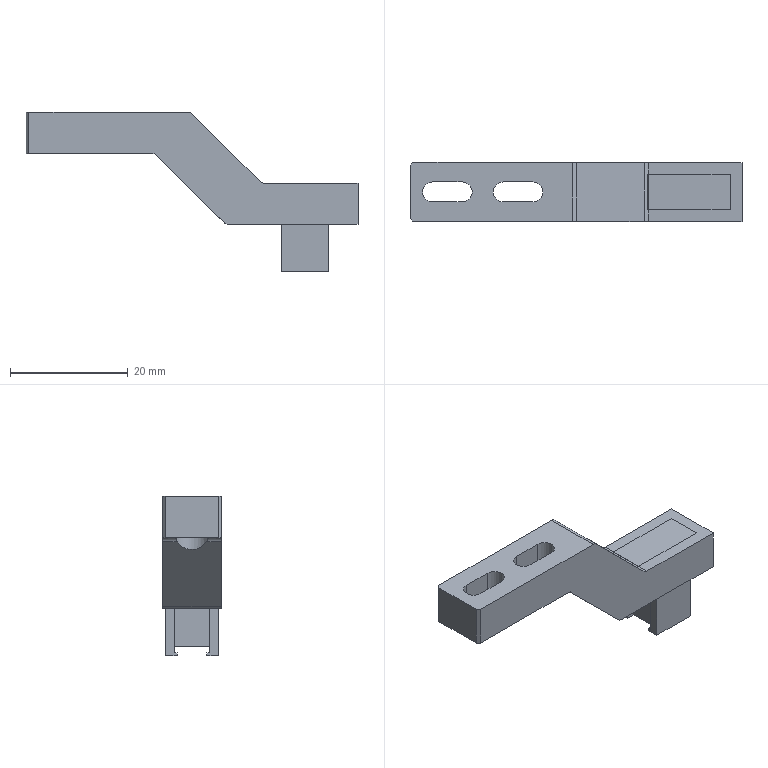NC program | NX | posted with a generic post | part box 56.3 x 10 x 27 mm
Lines 1 to 981 of 3920:
N10 G17 G21 G94 G90
(FLOOR_WALL_COPY , TOOL : D63)
N12 T01 M6
N14 G54
N16 G17 G0 G90 X62.65 Y0. S6500 M3
N18 G43 Z30. H1
N20 Z5.
N22 G94 G1 Z2. F1250.
N24 X59.65
N26 X-59.65
N28 X-62.65
N30 Z5.
N32 G0 Z30.
N34 X62.65
N36 Z4.
N38 G1 Z1.
N40 X59.65
N42 X-59.65
N44 X-62.65
N46 Z4.
N48 G0 Z30.
N50 X62.65
N52 Z3.
N54 G1 Z0.
N56 X59.65
N58 X-59.65
N60 X-62.65
N62 Z3.
N64 G0 Z30.
N66 M5
(ADAPTIVE_MILLING_COPY , TOOL : D10)
N68 T10 M6
N70 G54
N72 G17 G0 G90 X-29.095 Y-12.49 S9500 M3
N74 G43 Z30. H10
N76 Z-19.
N78 G94 G1 Z-20. F1000.
N80 X-28.723 Y-11.01 F3000.
N82 G3 X-29.383 Y-9.805 R1.015
N84 G2 X-31.661 Y-8.267 R5.47
N86 G1 X-32.538 Y-7.171
N88 X-32.612 Y-7.045
N90 X-32.995 Y-6.121
N92 G3 X-34.101 Y-5.513 R1.017
N94 G1 X-35.635 Y-5.779
N96 Z-17.
N98 G0 Z30.
N100 X-35.645 Y5.809
N102 Z-19.
N104 G1 Z-20. F1000.
N106 X-34.099 Y5.532 F3000.
N108 G3 X-32.988 Y6.14 R1.017
N110 G1 X-32.612 Y7.046
N112 X-32.539 Y7.17
N114 G2 X-30.75 Y9.106 R10.067
N116 X-29.382 Y9.805 R5.529
N118 G3 X-28.721 Y11.01 R1.015
N120 G1 X-29.093 Y12.485
N122 Z-17.
N124 G0 Z30.
N126 X-7.082 Y-12.562
N128 Z-18.85
N130 G1 Z-19.85 F1000.
N132 X-6.916 Y-11.769 F3000.
N134 X-6.774 Y-10.97
N136 G3 X-7.457 Y-9.975 R1.017
N138 X-11.391 Y-9.343 R13.467
N140 X-25.489 Y-9.186 R390.39
N142 G2 X-30.036 Y-6.459 R5.899
N144 X-31.966 Y-0.735 R12.739
N146 X-32.139 Y2.952 R16.321
N148 X-29.051 Y7.174 R6.209
N150 X-23.245 Y8.879 R13.977
N152 X-12.954 Y9.183 R112.101
N154 G3 X-9.257 Y9.221 R59.444
N156 G2 X-7.427 Y9.998 R15.276
N158 G3 X-7.037 Y11.746 R1.002
N160 X-7.789 Y11.981 Z-19.81 R1.212
N162 G1 X-8.981 Y12.072 Z-19.75
N164 X-11.324 Y12.248
N166 X-19.449
N168 G3 X-25.626 Y11.575 R29.031
N170 G1 X-26.698 Y11.337
N172 X-27.758 Y11.048
N174 G3 X-30.519 Y9.807 R13.655
N176 G1 X-32.085 Y8.865
N178 G3 X-33.546 Y7.281 R4.683
N180 G1 X-34.64 Y5.273
N182 G3 X-35.27 Y2.811 R6.964
N184 X-35.265 Y0.821 R11.97
N186 G1 X-35.027 Y-1.664
N188 G3 X-32.575 Y-7.973 R14.447
N190 G1 X-31.861 Y-8.997
N192 X-31.107 Y-9.991
N194 G3 X-30.156 Y-10.765 R3.251
N196 X-27.286 Y-11.946 R11.99
N198 X-24.825 Y-12.314 R13.023
N200 G1 X-11.112 Y-12.996
N202 X-10.881 Y-12.977
N204 X-10.659 Y-12.912
N206 X-8.91 Y-12.142
N208 X-8.301 Y-11.879 Z-19.783
N210 X-7.702 Y-11.595 Z-19.816
N212 G3 X-7.302 Y-11.069 Z-19.85 R1.04
N214 X-7.93 Y-9.814 R1.005
N216 G2 X-9.405 Y-9.206 R53.931
N218 G3 X-14.448 Y-8.54 R21.088
N220 X-23.346 Y-8.378 R966.397
N222 G2 X-29.253 Y-4.402 R7.758
N224 X-30.713 Y0.018 R9.774
N226 X-27.658 Y5.685 R6.887
N228 X-21.61 Y7.889 R13.615
N230 X-13.229 Y8.35 R64.733
N232 G3 X-10.141 Y8.517 R15.214
N234 X-8.908 Y9.377 R10.818
N236 X-8.643 Y10.699 R1.005
N238 X-9.549 Y11.199 Z-19.796 R1.107
N240 G1 X-10.461 Y11.321 Z-19.75
N242 X-12.805 Y11.627
N244 X-16.819 Y11.613
N246 G3 X-22.105 Y10.949 R28.919
N248 G1 X-24.626 Y10.376
N250 G3 X-29.545 Y8.323 R20.292
N252 X-32.51 Y5.291 R8.578
N254 X-33.55 Y2.864 R10.425
N256 X-33.946 Y1.048 R9.738
N258 X-33.405 Y-2.601 R8.322
N260 G1 X-32.84 Y-4.095
N262 X-32.26 Y-5.583
N264 G3 X-30.444 Y-8.234 R8.852
N266 X-29.053 Y-9.465 R9.477
N268 G1 X-28.528 Y-9.786
N270 X-27.98 Y-10.064
N272 G3 X-25.183 Y-11.114 R24.495
N274 X-23.224 Y-11.415 R8.92
N276 G1 X-12.474 Y-11.804
N278 X-12.318 Y-11.798
N280 X-10.15 Y-11.536
N282 X-9.486 Y-11.46 Z-19.783
N284 X-8.825 Y-11.362 Z-19.817
N286 G3 X-8.294 Y-10.985 Z-19.85 R1.041
N288 X-8.577 Y-9.554 R1.004
N290 X-12.565 Y-8.09 R8.471
N292 X-20.747 Y-7.642 R67.984
N294 G2 X-28.031 Y-3.29 R8.284
N296 X-27.114 Y3.185 R6.128
N298 X-21.759 Y6.499 R10.353
N300 X-14.338 Y7.453 R31.44
N302 G3 X-10.767 Y7.816 R15.161
N304 X-9.893 Y8.632 R2.14
N306 G1 X-9.821 Y8.701
N308 G3 X-9.629 Y9.891 R1.007
N310 X-10.436 Y10.425 Z-19.8 R1.037
N312 G1 X-11.413 Y10.597 Z-19.75
N314 X-13.396 Y10.947
N316 X-13.557 Y10.958
N318 X-13.718 Y10.951
N320 X-21.538 Y9.776
N322 G3 X-25.619 Y8.334 R11.544
N324 X-30.189 Y4.197 R14.319
N326 G1 X-30.651 Y3.515
N328 X-31.071 Y2.807
N330 G3 X-31.699 Y-0.315 R5.897
N332 G1 X-31.595 Y-1.716
N334 X-31.471 Y-3.116
N336 G3 X-30.853 Y-4.752 R4.789
N338 G1 X-30.104 Y-5.877
N340 X-29.329 Y-6.984
N342 G3 X-27.033 Y-8.977 R8.046
N344 X-23.3 Y-10.28 R10.192
N346 X-17.104 Y-10.992 R86.895
N348 G1 X-13.208 Y-11.279
N350 X-11.031 Y-10.969
N352 X-10.377 Y-10.88 Z-19.783
N354 X-9.728 Y-10.766 Z-19.816
N356 G3 X-9.198 Y-10.359 Z-19.85 R1.039
N358 X-9.42 Y-9.027 R1.005
N360 X-12.364 Y-7.611 R5.895
N362 X-19.018 Y-6.918 R38.53
N364 G2 X-23.754 Y-5.513 R9.337
N366 X-25.428 Y0.573 R5.13
N368 X-21.1 Y4.933 R8.141
N370 X-15.011 Y6.433 R19.241
N372 G3 X-11.371 Y7.051 R17.404
N374 X-10.667 Y7.667 R1.259
N376 G1 X-10.292 Y8.135
N378 G3 X-10.2 Y9.25 R1.01
N380 X-10.945 Y9.757 Z-19.803 R1.047
N382 G1 X-11.986 Y9.994 Z-19.75
N384 X-12.93 Y10.215
N386 X-13.879 Y10.412
N388 X-14.189 Y10.385
N390 X-17.418 Y9.565
N392 G3 X-23.015 Y7.362 R30.115
N394 X-25.904 Y5.324 R13.843
N396 X-27.531 Y3.25 R9.668
N398 G1 X-28.137 Y2.209
N400 X-28.726 Y1.158
N402 G3 X-29.135 Y-1.686 R4.979
N404 X-28.711 Y-3.27 R6.554
N406 G1 X-28.229 Y-4.44
N408 X-27.73 Y-5.603
N410 G3 X-24.517 Y-8.671 R6.669
N412 X-22.152 Y-9.426 R10.665
N414 G1 X-13.426 Y-11.085
N416 X-13.181 Y-11.071
N418 X-11.297 Y-10.727
N420 X-10.648 Y-10.614 Z-19.783
N422 X-10.003 Y-10.477 Z-19.816
N424 G3 X-9.489 Y-10.05 Z-19.85 R1.039
N426 X-9.651 Y-8.82 R1.007
N428 X-12.954 Y-6.968 R6.175
N430 X-18.092 Y-6.206 R37.578
N432 G2 X-21.119 Y-4.858 R4.47
N434 X-21.743 Y0.226 R4.837
N436 X-17.592 Y4.231 R8.054
N438 X-12.947 Y5.775 R33.71
N440 G3 X-11.176 Y6.658 R4.145
N442 X-10.738 Y7.55 R7.192
N444 X-10.92 Y8.632 R1.01
N446 X-11.892 Y8.942 Z-19.797 R1.115
N448 G1 X-12.828 Y8.893 Z-19.75
N450 X-14.861 Y8.78
N452 X-15.085 Y8.715
N454 G3 X-20.073 Y6.318 R44.561
N456 X-23.345 Y3.452 R11.589
N458 G1 X-24.168 Y2.369
N460 G3 X-25.085 Y-0.66 R5.509
N462 X-23.769 Y-5.511 R9.449
N464 X-21.913 Y-7.647 R9.299
N466 X-17.768 Y-9.753 R8.705
N468 G1 X-15.897 Y-10.136
N470 X-14.022 Y-10.496
N472 X-13.749 Y-10.475
N474 X-11.973 Y-10.091
N476 X-11.316 Y-9.953 Z-19.784
N478 X-10.664 Y-9.793 Z-19.817
N480 G3 X-10.173 Y-9.374 Z-19.85 R1.041
N482 X-10.261 Y-8.229 R1.007
N484 X-12.616 Y-6.595 R4.561
N486 X-15.415 Y-5.848 R27.634
N488 G2 X-17.591 Y-2.639 R3.565
N490 X-15.665 Y2.136 R6.397
N492 X-12.32 Y4.826 R24.044
N494 G3 X-11.366 Y5.826 R2.693
N496 G2 X-11.035 Y6.875 R3.828
N498 G3 X-11.436 Y8.135 R1.005
N500 X-12.403 Y8.175 Z-19.8 R1.037
N502 G1 X-13.328 Y7.818 Z-19.75
N504 X-14.324 Y7.438
N506 X-15.314 Y7.042
N508 X-15.535 Y6.875
N510 X-16.742 Y5.673
N512 X-17.934 Y4.456
N514 G3 X-19.803 Y1.357 R9.754
N516 G1 X-20.095 Y0.566
N518 X-20.341 Y-0.241
N520 G3 X-20.431 Y-2.92 R6.368
N522 X-19.976 Y-4.243 R5.551
N524 G1 X-19.325 Y-5.556
N526 X-18.653 Y-6.859
N528 G3 X-16.386 Y-8.672 R4.213
N530 G1 X-14.631 Y-9.247
N532 X-12.462 Y-9.477
N534 X-11.811 Y-9.549 Z-19.783
N536 X-11.159 Y-9.596 Z-19.816
N538 G3 X-10.539 Y-9.323 Z-19.85 R1.038
N540 X-10.39 Y-8.054 R1.007
N542 X-12.253 Y-6.296 R4.463
N544 G2 X-14.109 Y-1.889 R4.864
N546 X-12.538 Y2.385 R9.455
N548 G3 X-11.5 Y4.204 R10.631
N550 G2 X-11.315 Y6.023 R12.347
N552 G3 X-12.598 Y7.131 R1.002
N554 X-13.233 Y6.59 Z-19.807 R1.173
N556 G1 X-13.887 Y5.65 Z-19.75
N558 X-15.152 Y3.839
N560 X-15.821 Y3.15
N562 G3 X-16.324 Y2.308 R3.162
N564 X-17.074 Y-0.188 R11.037
N566 G1 X-17.333 Y-2.504
N568 X-17.567 Y-4.822
N570 G3 X-16.464 Y-6.889 R2.105
N572 G1 X-15.156 Y-7.58
N574 X-13.093 Y-8.503
N576 X-12.46 Y-8.789 Z-19.785
N578 X-11.82 Y-9.059 Z-19.82
N580 G3 X-11.22 Y-9.037 Z-19.85 R1.047
N582 X-10.716 Y-7.551 R1.003
N584 G2 X-12.171 Y-4.447 R9.788
N586 X-11.741 Y0.772 R10.008
N588 G3 X-11.396 Y2.055 R6.869
N590 G2 X-11.474 Y4.376 R17.958
N592 G3 X-13.672 Y4.322 R-1.1
N594 G1 X-13.081 Y-7.6
N596 G3 X-10.95 Y-7.167 R-1.1
N598 G2 X-11.474 Y-4.966 R6.015
N600 X-10.997 Y0.064 R17.199
N602 G3 X-11.006 Y0.742 R1.809
N604 G2 X-11.401 Y2.103 R3.769
N606 G3 X-13.596 Y1.974 R1.1
N608 G1 X-13.529 Y-1.466
N610 G3 X-11.359 Y-1.699 R1.1
N612 G1 X-11.326 Y-1.56
N614 X-10.929 Y-0.538
N616 X-10.891 Y-0.419
N618 X-10.849 Y-0.257
N620 G3 X-11.04 Y0.83 R1.782
N622 X-12.218 Y1.443 R1.015
N624 G1 X-13.775 Y1.068
N626 Z-16.85
N628 G0 Z30.
N630 X-6.934 Y-12.51
N632 Z-18.403
N634 G1 Z-19.403 F1000.
N636 X-6.755 Y-11.705 F3000.
N638 X-6.598 Y-10.895
N640 G3 X-7.221 Y-9.903 R1.017
N642 G2 X-10.204 Y-7.513 R5.363
N644 X-10.871 Y-4.965 R6.053
N646 X-10.737 Y-1.404 R21.01
N648 G3 X-10.761 Y1.513 R4.162
N650 G2 X-10.703 Y6.266 R17.594
N652 X-8.225 Y9.488 R5.424
N654 G1 X-7.116 Y9.946
N656 G3 X-7.6 Y11.865 R1.
N658 G1 X-9.58 Y11.582 Z-19.303
N660 X-10.319 Y11.482
N662 X-11.054 Y11.358
N664 X-11.271 Y11.256
N666 X-11.462 Y11.111
N668 X-11.902 Y10.672
N670 X-12.298 Y10.194
N672 X-12.456 Y9.929
N674 X-12.597 Y9.655
N676 X-13.458 Y7.659
N678 G3 X-14.312 Y3.881 R13.264
N680 G1 X-14.508 Y1.226
N682 G3 X-14.201 Y0.429 R1.016
N684 G1 X-13.127 Y-0.596
N686 X-12.634 Y-1.071 Z-19.337
N688 X-12.128 Y-1.532 Z-19.372
N690 G3 X-11.533 Y-1.709 Z-19.403 R1.044
N692 X-10.61 Y-1.024 R1.007
N694 X-10.397 Y0.36 R2.262
N696 G1 X-10.426 Y0.468
N698 X-10.584 Y0.942
N700 G3 X-11.815 Y1.596 R1.015
N702 G1 X-13.23 Y1.199
N704 Z-16.403
N706 G0 Z30.
N708 X-5.663 Y-12.6
N710 Z-17.806
N712 G1 Z-18.806 F1000.
N714 X-5.955 Y-10.725 F3000.
N716 G3 X-6.572 Y-9.945 R1.024
N718 G2 X-10.178 Y-6.271 R5.329
N720 G1 X-10.348 Y-5.036
N722 X-10.353 Y-4.964
N724 G2 X-10.256 Y-1.202 R28.314
N726 G3 X-10.269 Y1.277 R3.928
N728 G2 X-10.348 Y5.036 R30.281
N730 X-8.856 Y8.6 R5.576
N732 X-6.562 Y9.95 R5.798
N734 G3 X-7.063 Y11.868 R1.
N736 G1 X-9.043 Y11.584 Z-18.706
N738 X-9.773 Y11.484
N740 X-10.5 Y11.362
N742 X-10.717 Y11.26
N744 X-10.908 Y11.114
N746 X-11.348 Y10.675
N748 X-11.745 Y10.198
N750 X-11.904 Y9.934
N752 X-12.047 Y9.66
N754 X-12.953 Y7.59
N756 G3 X-13.817 Y3.884 R13.572
N758 G1 X-14.011 Y1.631
N760 G3 X-13.722 Y0.837 R1.024
N762 G1 X-12.634 Y-0.25
N764 X-12.16 Y-0.731 Z-18.74
N766 X-11.67 Y-1.196 Z-18.774
N768 G3 X-11.061 Y-1.383 Z-18.806 R1.042
N770 X-10.114 Y-0.619 R1.007
N772 X-10.072 Y0.442 R1.7
N774 X-11.066 Y1.213 R1.017
N776 G1 X-12.768 Y1.192
N778 Z-15.806
N780 G0 Z30.
N782 X-5.041 Y-12.603
N784 Z-17.21
N786 G1 Z-18.21 F1000.
N788 X-5.339 Y-10.729 F3000.
N790 G3 X-5.955 Y-9.952 R1.024
N792 G2 X-9.07 Y-7.522 R5.482
N794 X-9.753 Y-4.964 R6.077
N796 G1 Y-1.39
N798 X-9.75 Y-1.332
N800 G3 X-9.753 Y1.306 R7.407
N802 G1 Y4.964
N804 X-9.748 Y5.036
N806 G2 X-8.256 Y8.6 R5.576
N808 X-5.948 Y9.955 R5.84
N810 G3 X-6.456 Y11.873 R1.
N812 G1 X-8.436 Y11.588 Z-18.11
N814 X-9.163 Y11.489
N816 X-9.886 Y11.367
N818 X-10.103 Y11.265
N820 X-10.295 Y11.12
N822 X-11.04 Y10.378
N824 X-11.772 Y9.624
N826 G3 X-12.809 Y6.852 R4.345
N828 G1 X-12.835 Y2.52
N830 X-12.774 Y2.276
N832 X-12.234 Y0.883
N834 X-11.543 Y-0.882 Z-18.204
N836 X-11.491 Y-0.972 Z-18.21
N838 G3 X-9.66 Y-0.537 R1.001
N840 X-9.626 Y0.221 R7.411
N842 X-10.714 Y1.107 R1.015
N844 G1 X-12.235 Y0.978
N846 Z-15.21
N848 G0 Z30.
N850 X-4.441 Y-12.603
N852 Z-16.613
N854 G1 Z-17.613 F1000.
N856 X-4.739 Y-10.729 F3000.
N858 G3 X-5.355 Y-9.952 R1.024
N860 G2 X-8.47 Y-7.522 R5.482
N862 X-9.153 Y-4.964 R6.077
N864 G1 Y4.964
N866 X-9.148 Y5.036
N868 G2 X-7.656 Y8.6 R5.576
N870 X-5.348 Y9.955 R5.84
N872 G3 X-4.738 Y11.085 R1.017
N874 G1 X-5.02 Y12.525
N876 Z-14.613
N878 G0 Z30.
N880 X-3.841 Y-12.603
N882 Z-16.016
N884 G1 Z-17.016 F1000.
N886 X-4.139 Y-10.729 F3000.
N888 G3 X-4.755 Y-9.952 R1.024
N890 G2 X-7.87 Y-7.522 R5.482
N892 X-8.553 Y-4.964 R6.077
N894 G1 Y4.964
N896 X-8.548 Y5.036
N898 G2 X-7.056 Y8.599 R5.576
N900 X-4.748 Y9.955 R5.84
N902 G3 X-4.138 Y11.085 R1.017
N904 G1 X-4.42 Y12.525
N906 Z-14.016
N908 G0 Z30.
N910 X-3.241 Y-12.603
N912 Z-15.419
N914 G1 Z-16.419 F1000.
N916 X-3.539 Y-10.729 F3000.
N918 G3 X-4.155 Y-9.952 R1.024
N920 G2 X-7.27 Y-7.522 R5.481
N922 X-7.953 Y-4.964 R6.077
N924 G1 Y4.964
N926 X-7.948 Y5.036
N928 G2 X-6.456 Y8.6 R5.576
N930 X-4.147 Y9.955 R5.84
N932 G3 X-3.537 Y11.085 R1.017
N934 G1 X-3.819 Y12.525
N936 Z-13.419
N938 G0 Z30.
N940 X-2.641 Y-12.603
N942 Z-14.823
N944 G1 Z-15.823 F1000.
N946 X-2.939 Y-10.729 F3000.
N948 G3 X-3.555 Y-9.952 R1.024
N950 G2 X-6.67 Y-7.522 R5.481
N952 X-7.352 Y-4.964 R6.077
N954 G1 Y4.964
N956 X-7.348 Y5.036
N958 G2 X-5.856 Y8.599 R5.576
N960 X-3.547 Y9.955 R5.84
N962 G3 X-2.937 Y11.085 R1.017
N964 G1 X-3.219 Y12.525
N966 Z-12.823
N968 G0 Z30.
N970 X-2.042 Y-12.603
N972 Z-14.226
N974 G1 Z-15.226 F1000.
N976 X-2.339 Y-10.729 F3000.
N978 G3 X-2.955 Y-9.952 R1.024
N980 G2 X-6.07 Y-7.522 R5.481
N982 X-6.752 Y-4.964 R6.077
N984 G1 Y4.964
N986 X-6.747 Y5.036
N988 G2 X-5.256 Y8.599 R5.576
N990 X-2.947 Y9.955 R5.84
N992 G3 X-2.337 Y11.085 R1.017
N994 G1 X-2.619 Y12.525
N996 Z-12.226
N998 G0 Z30.
N1000 X-1.442 Y-12.603
N1002 Z-13.629
N1004 G1 Z-14.629 F1000.
N1006 X-1.739 Y-10.729 F3000.
N1008 G3 X-2.355 Y-9.952 R1.024
N1010 G2 X-5.469 Y-7.522 R5.481
N1012 X-6.152 Y-4.964 R6.077
N1014 G1 Y4.964
N1016 X-6.147 Y5.036
N1018 G2 X-4.655 Y8.599 R5.576
N1020 X-2.347 Y9.955 R5.84
N1022 G3 X-1.737 Y11.085 R1.017
N1024 G1 X-2.019 Y12.525
N1026 Z-11.629
N1028 G0 Z30.
N1030 X-0.842 Y-12.603
N1032 Z-13.032
N1034 G1 Z-14.032 F1000.
N1036 X-1.139 Y-10.729 F3000.
N1038 G3 X-1.755 Y-9.952 R1.024
N1040 G2 X-4.869 Y-7.522 R5.48
N1042 X-5.552 Y-4.964 R6.077
N1044 G1 Y4.964
N1046 X-5.547 Y5.036
N1048 G2 X-4.055 Y8.599 R5.576
N1050 X-1.747 Y9.955 R5.84
N1052 G3 X-1.137 Y11.085 R1.017
N1054 G1 X-1.419 Y12.525
N1056 Z-11.032
N1058 G0 Z30.
N1060 X-0.242 Y-12.603
N1062 Z-12.435
N1064 G1 Z-13.435 F1000.
N1066 X-0.539 Y-10.729 F3000.
N1068 G3 X-1.155 Y-9.952 R1.024
N1070 G2 X-4.269 Y-7.522 R5.48
N1072 X-4.952 Y-4.964 R6.077
N1074 G1 Y4.964
N1076 X-4.947 Y5.036
N1078 G2 X-3.455 Y8.6 R5.576
N1080 X-1.147 Y9.955 R5.84
N1082 G3 X-0.537 Y11.085 R1.017
N1084 G1 X-0.819 Y12.525
N1086 Z-10.435
N1088 G0 Z30.
N1090 X0.358 Y-12.603
N1092 Z-11.839
N1094 G1 Z-12.839 F1000.
N1096 X0.061 Y-10.729 F3000.
N1098 G3 X-0.555 Y-9.952 R1.024
N1100 G2 X-3.669 Y-7.522 R5.48
N1102 X-4.352 Y-4.964 R6.077
N1104 G1 Y4.964
N1106 X-4.347 Y5.036
N1108 G2 X-2.855 Y8.599 R5.576
N1110 X-0.547 Y9.955 R5.84
N1112 G3 X0.063 Y11.085 R1.017
N1114 G1 X-0.219 Y12.525
N1116 Z-9.839
N1118 G0 Z30.
N1120 X0.958 Y-12.603
N1122 Z-11.242
N1124 G1 Z-12.242 F1000.
N1126 X0.661 Y-10.729 F3000.
N1128 G3 X0.045 Y-9.952 R1.024
N1130 G2 X-3.069 Y-7.522 R5.48
N1132 X-3.752 Y-4.964 R6.077
N1134 G1 Y4.964
N1136 X-3.747 Y5.036
N1138 G2 X-2.255 Y8.599 R5.576
N1140 X0.053 Y9.955 R5.84
N1142 G3 X0.664 Y11.085 R1.017
N1144 G1 X0.381 Y12.525
N1146 Z-9.242
N1148 G0 Z30.
N1150 X1.558 Y-12.603
N1152 Z-10.645
N1154 G1 Z-11.645 F1000.
N1156 X1.261 Y-10.729 F3000.
N1158 G3 X0.645 Y-9.951 R1.024
N1160 G2 X-2.469 Y-7.522 R5.479
N1162 X-3.151 Y-4.964 R6.077
N1164 G1 Y4.964
N1166 X-3.147 Y5.036
N1168 G2 X-1.655 Y8.6 R5.576
N1170 X0.654 Y9.955 R5.84
N1172 G3 X1.264 Y11.085 R1.017
N1174 G1 X0.982 Y12.525
N1176 Z-8.645
N1178 G0 Z30.
N1180 X2.158 Y-12.603
N1182 Z-10.048
N1184 G1 Z-11.048 F1000.
N1186 X1.861 Y-10.729 F3000.
N1188 G3 X1.245 Y-9.951 R1.024
N1190 G2 X-1.869 Y-7.522 R5.479
N1192 X-2.551 Y-4.964 R6.077
N1194 G1 Y4.964
N1196 X-2.546 Y5.036
N1198 G2 X-1.055 Y8.599 R5.576
N1200 X1.254 Y9.955 R5.84
N1202 G3 X1.864 Y11.085 R1.017
N1204 G1 X1.582 Y12.525
N1206 Z-8.048
N1208 G0 Z30.
N1210 X2.758 Y-12.603
N1212 Z-9.452
N1214 G1 Z-10.452 F1000.
N1216 X2.461 Y-10.729 F3000.
N1218 G3 X1.845 Y-9.951 R1.024
N1220 G2 X-1.268 Y-7.522 R5.479
N1222 X-1.951 Y-4.964 R6.077
N1224 G1 Y4.964
N1226 X-1.946 Y5.036
N1228 G2 X-0.454 Y8.599 R5.576
N1230 X1.854 Y9.955 R5.84
N1232 G3 X2.464 Y11.085 R1.017
N1234 G1 X2.182 Y12.525
N1236 Z-7.452
N1238 G0 Z30.
N1240 X3.358 Y-12.603
N1242 Z-8.855
N1244 G1 Z-9.855 F1000.
N1246 X3.061 Y-10.729 F3000.
N1248 G3 X2.445 Y-9.951 R1.024
N1250 G2 X-0.668 Y-7.522 R5.479
N1252 X-1.351 Y-4.964 R6.077
N1254 G1 Y4.964
N1256 X-1.346 Y5.036
N1258 G2 X0.146 Y8.599 R5.576
N1260 X2.454 Y9.955 R5.84
N1262 G3 X3.064 Y11.085 R1.017
N1264 G1 X2.782 Y12.525
N1266 Z-6.855
N1268 G0 Z30.
N1270 X3.958 Y-12.603
N1272 Z-8.258
N1274 G1 Z-9.258 F1000.
N1276 X3.661 Y-10.728 F3000.
N1278 G3 X3.045 Y-9.951 R1.024
N1280 G2 X-0.068 Y-7.522 R5.478
N1282 X-0.751 Y-4.964 R6.077
N1284 G1 Y4.964
N1286 X-0.746 Y5.036
N1288 G2 X0.746 Y8.599 R5.576
N1290 X3.054 Y9.955 R5.84
N1292 G3 X3.664 Y11.085 R1.017
N1294 G1 X3.382 Y12.525
N1296 Z-6.258
N1298 G0 Z30.
N1300 X4.558 Y-12.603
N1302 Z-7.661
N1304 G1 Z-8.661 F1000.
N1306 X4.261 Y-10.728 F3000.
N1308 G3 X3.645 Y-9.951 R1.024
N1310 G2 X0.532 Y-7.522 R5.478
N1312 X-0.151 Y-4.964 R6.077
N1314 G1 Y4.964
N1316 X-0.146 Y5.036
N1318 G2 X1.346 Y8.599 R5.576
N1320 X3.654 Y9.955 R5.84
N1322 G3 X4.264 Y11.085 R1.017
N1324 G1 X3.982 Y12.525
N1326 Z-5.661
N1328 G0 Z30.
N1330 X5.262 Y-12.603
N1332 Z-7.065
N1334 G1 Z-8.065 F1000.
N1336 X4.96 Y-10.736 F3000.
N1338 G3 X4.336 Y-9.958 R1.024
N1340 G2 X1.183 Y-7.539 R5.517
N1342 X0.471 Y-4.962 R6.121
N1344 G1 Y4.962
N1346 X0.476 Y5.038
N1348 G2 X2.014 Y8.618 R5.626
N1350 X4.354 Y9.966 R5.899
N1352 G3 X4.973 Y11.094 R1.017
N1354 G1 X4.699 Y12.532
N1356 Z-5.065
N1358 G0 Z30.
N1360 X35.844 Y0.047
N1362 Z-6.85
N1364 G1 Z-7.85 F1000.
N1366 X34.488 Y0.577 F3000.
N1368 G3 X33.197 Y0.047 R1.015
N1370 X32.55 Y-3.011 R9.779
N1372 G2 X29.42 Y-7.204 R6.244
N1374 X26.468 Y-8.415 R13.151
N1376 X23.184 Y-9.646 R5.534
N1378 G1 X23.116 Y-9.65
N1380 X15.184
N1382 X15.116 Y-9.646
N1384 G3 X7.894 Y-9.22 R54.184
N1386 G2 X3.584 Y-6.443 R5.975
N1388 X1.717 Y-0.902 R12.783
N1390 X1.502 Y2.884 R18.485
N1392 X4.629 Y7.189 R6.193
N1394 X10.24 Y8.86 R13.889
N1396 G3 X12.927 Y9.106 R67.672
N1398 G2 X15.184 Y9.65 R5.627
N1400 G1 X23.116
N1402 X23.184 Y9.646
N1404 X24.415 Y9.484
N1406 X24.713 Y9.451
N1408 X25.012 Y9.422
N1410 X25.311 Y9.397
N1412 X25.51 Y9.382
N1414 X25.809 Y9.361
N1416 X25.909 Y9.352
N1418 X26.008 Y9.34
N1420 X26.107 Y9.326
N1422 X26.206 Y9.31
N1424 X26.304 Y9.292
N1426 X26.402 Y9.272
N1428 G2 X30.525 Y5.886 R6.471
N1430 X31.749 Y0.483 R11.107
N1432 X29.005 Y-5.282 R7.471
N1434 G3 X27.976 Y-6.225 R7.956
N1436 G2 X26.34 Y-8.488 R4.793
N1438 G1 X26.009 Y-8.749
N1440 X25.661 Y-8.986
N1442 G2 X23.116 Y-9.65 R6.123
N1444 G1 X15.116 Y-9.646
N1446 X13.885 Y-9.484
N1448 G3 X10.06 Y-8.631 R12.982
N1450 G2 X4.212 Y-4.216 R8.172
N1452 X2.918 Y-0.046 R10.199
N1454 X5.934 Y5.643 R6.897
N1456 X10.684 Y7.672 R13.311
N1458 G3 X11.563 Y8.183 R1.456
N1460 G2 X13.008 Y9.139 R5.18
N1462 G3 X12.735 Y11.057 R1.001
N1464 G1 X12.433 Y11.044 Z-7.835
N1466 X12.135 Y10.985 Z-7.82
N1468 X10.77 Y10.709 Z-7.75
N1470 X8.761 Y10.309
N1472 X7.116 Y10.29
N1474 G3 X5.278 Y9.42 R3.052
N1476 G1 X3.951 Y8.098
N1478 X2.639 Y6.761
N1480 G3 X0.836 Y4.243 R13.608
N1482 G1 X0.094 Y2.872
N1484 G3 X-0.228 Y0.748 R4.316
N1486 G1 X0.005 Y-1.663
N1488 G3 X1.591 Y-6.088 R11.724
N1490 X5.278 Y-10.045 R12.225
N1492 X7.934 Y-11.513 R15.203
N1494 G1 X10.11 Y-12.439
N1496 G3 X10.987 Y-12.393 R1.016
N1498 G1 X12.391 Y-11.612
N1500 X12.97 Y-11.297 Z-7.783
N1502 X13.536 Y-10.96 Z-7.816
N1504 G3 X13.887 Y-10.39 Z-7.85 R1.039
N1506 X13.292 Y-9.257 R1.007
N1508 X10.037 Y-7.865 R65.182
N1510 G2 X5.232 Y-2.998 R9.334
N1512 X6.805 Y3.652 R6.484
N1514 X10.13 Y6.199 R18.265
N1516 G3 X10.732 Y7.13 R2.195
N1518 G1 X11.462 Y8.082
N1520 G3 X10.994 Y9.636 R1.003
N1522 X10.09 Y9.529 Z-7.803 R1.151
N1524 G1 X9.117 Y9.102 Z-7.75
N1526 X7.158 Y8.234
N1528 X6.962 Y8.082
N1530 X4.322 Y5.424
N1532 G3 X2.247 Y2.597 R15.225
N1534 X1.579 Y-0.522 R6.004
N1536 X2.395 Y-4.132 R11.571
N1538 X3.312 Y-6.032 R10.736
N1540 X5.174 Y-8.197 R12.039
N1542 G1 X6.892 Y-9.69
N1544 X8.623 Y-11.168
N1546 G3 X9.529 Y-11.375 R1.015
N1548 G1 X11.067 Y-10.969
N1550 X11.702 Y-10.807 Z-7.783
N1552 X12.329 Y-10.62 Z-7.816
N1554 G3 X12.812 Y-10.147 Z-7.85 R1.038
N1556 X12.52 Y-8.918 R1.007
N1558 G2 X9.186 Y-6.357 R78.766
N1560 X7.65 Y1.011 R6.158
N1562 X9.876 Y4.441 R17.802
N1564 G3 X10.167 Y5.765 R3.317
N1566 G1 X10.202 Y5.897
N1568 X10.508 Y6.636
N1570 G3 X9.68 Y8.014 R1.003
N1572 X8.815 Y7.686 Z-7.802 R1.142
N1574 G1 X7.994 Y7.038 Z-7.75
N1576 X7.155 Y6.382
N1578 X6.329 Y5.71
N1580 X6.161 Y5.471
N1582 X5.345 Y3.847
N1584 X4.548 Y2.213
N1586 G3 X3.712 Y-2.905 R10.306
N1588 X5.145 Y-6.541 R7.651
N1590 G1 X7.216 Y-9.348
N1592 G3 X7.973 Y-9.753 R1.016
N1594 G1 X9.654 Y-9.834
N1596 X10.315 Y-9.871 Z-7.783
N1598 X10.977 Y-9.883 Z-7.816
N1600 G3 X11.571 Y-9.589 Z-7.85 R1.039
N1602 X11.563 Y-8.183 R1.005
N1604 G2 X9.611 Y-5.488 R16.919
N1606 X9.331 Y0.453 R7.881
N1608 G3 X10. Y2.474 R35.275
N1610 G2 X10.044 Y4.832 R23.284
N1612 G3 X7.857 Y4.883 R-1.1
N1614 G1 X8.95 Y-8.135
N1616 G3 X10.919 Y-7.373 R-1.1
N1618 G2 X10.005 Y-4.534 R5.185
N1620 X10. Y-2.62 R23.649
N1622 G1 Y2.48
N1624 G3 X7.8 Y2.457 R-1.1
N1626 G1 X7.976 Y-5.931
N1628 G3 X10.167 Y-5.765 R-1.1
N1630 G1 X10. Y-4.466
N1632 Y-2.566
N1634 G3 X9.552 Y-1.732 R1.014
N1636 G1 X9.174 Y-1.481
N1638 X7.506 Y-0.377 Z-7.75
N1640 X7.25 Y-0.206
N1642 X7.026 Y0.005
N1644 G2 X6.818 Y0.616 R1.041
N1646 G1 X6.816 Y2.246
N1648 X6.832 Y3.876
N1650 G2 X7.702 Y7.75 R11.749
N1652 G1 X8.277 Y9.104
N1654 G2 X10.58 Y11.62 R5.959
N1656 X12.494 Y12.324 R6.935
N1658 X14.589 Y12.579 R12.491
N1660 X18.33 Y12.688 R54.349
N1662 G1 X21.233 Y12.665
N1664 G2 X22.101 Y12.167 R1.061
N1666 G1 X23.316 Y10.578 Z-7.85
N1668 X23.645 Y10.143
N1670 X23.989 Y9.72
N1672 X24.189 Y9.579
N1674 X24.415 Y9.484
N1676 G2 X28.179 Y6.823 R7.675
N1678 X30.181 Y0.802 R8.542
N1680 X28.595 Y-3.476 R10.68
N1682 G3 X28.296 Y-4.534 R1.635
N1684 G1 X28.134 Y-5.765
N1686 X28.098 Y-5.897
N1688 X27.907 Y-6.358
N1690 G3 X29.476 Y-7.505 R1.001
N1692 G1 X29.691 Y-7.258 Z-7.834
N1694 X29.874 Y-6.986 Z-7.817
N1696 X30.63 Y-5.875 Z-7.75
N1698 X31.758 Y-4.207
N1700 G3 X33.09 Y-0.599 R39.223
N1702 X33.334 Y1.842 R6.405
N1704 G1 X33.152 Y3.59
N1706 G3 X31.673 Y7.606 R10.585
N1708 G1 X30.126 Y10.083
N1710 G3 X29.333 Y10.552 R1.015
N1712 G1 X27.649 Y10.644
N1714 X26.967 Y10.686 Z-7.784
N1716 X26.285 Y10.706 Z-7.818
N1718 G3 X25.716 Y10.451 Z-7.85 R1.043
N1720 X25.78 Y8.918 R1.003
N1722 G2 X28.098 Y5.897 R5.486
N1724 X28.327 Y-0.864 R10.109
N1726 G1 X28.3 Y-4.233
N1728 G3 X30.5 Y-4.208 R-1.1
N1730 G1 X30.26 Y6.206
N1732 G3 X28.098 Y5.897 R-1.1
N1734 G1 X28.134 Y5.765
N1736 X28.296 Y4.534
N1738 X28.3 Y4.466
N1740 Y-1.034
N1742 G3 X28.527 Y-1.672 R1.049
N1744 G1 X30.8 Y-4.466
N1746 Z-4.85
N1748 G0 Z30.
N1750 M5
(FLOOR_WALL_1_1 , TOOL : D6)
N1752 T06 M6
N1754 G54
N1756 G17 G0 G90 X32.145 Y-9.123 S9500 M3
N1758 G43 Z30. H6
N1760 Z-6.5
N1762 G94 G1 Z-8. F1250.
N1764 X31.67 Y-8.3
N1766 G3 X31.15 Y-8. R0.6
N1768 G1 X3.14
N1770 Y-5.35
N1772 X11.85
N1774 Y-2.7
N1776 X3.14
N1778 Y-0.05
N1780 X11.85
N1782 Y2.6
N1784 X3.14
N1786 Y5.25
N1788 X11.85
N1790 Z-6.5
N1792 G0 Z30.
N1794 Y-5.35
N1796 Z-6.5
N1798 G1 Z-8.
N1800 Y-7.5
N1802 G3 X12.15 Y-7.8 R0.3
N1804 G1 X26.15
N1806 G3 X26.45 Y-7.5 R0.3
N1808 G1 Y-5.35
N1810 X31.15
N1812 Y-2.7
N1814 X26.45
N1816 Y-0.05
N1818 X31.15
N1820 Y2.6
N1822 X26.45
N1824 Y5.25
N1826 X31.15
N1828 Y7.9
N1830 X3.14
N1832 G3 X2.62 Y7.6 R0.6
N1834 G1 X1.64 Y5.902
N1836 Z-6.5
N1838 G0 Z30.
N1840 X10.35 Y-1.386
N1842 Z-6.5
N1844 G1 Z-8.
N1846 X11.85 Y-0.52
N1848 G3 X12.15 Y0. R0.6
N1850 G1 Y7.5
N1852 X26.15
N1854 Y-7.5
N1856 X12.15
N1858 Y0.
N1860 G3 X11.85 Y0.52 R0.6
N1862 G1 X10.35 Y1.386
N1864 Z-6.5
N1866 G0 Z30.
N1868 X-32.273 Y-6.737
N1870 Z-18.5
N1872 G1 Z-20.
N1874 X-31.45 Y-6.262
N1876 G3 X-31.15 Y-5.743 R0.6
N1878 G1 Y5.743
N1880 X-28.893 Y8.
N1882 X-28.496
N1884 Y-8.
N1886 X-25.842
N1888 Y8.
N1890 X-23.188
N1892 Y-8.
N1894 X-20.534
N1896 Y8.
N1898 X-17.881
N1900 Y-8.
N1902 X-15.227
N1904 Y8.
N1906 X-12.573
N1908 Y-8.
N1910 X-9.919
N1912 Y8.
N1914 G3 X-10.219 Y8.52 R0.6
N1916 G1 X-11.917 Y9.5
N1918 Z-18.5
N1920 G0 Z30.
N1922 X-11.617 Y-9.5
N1924 Z-18.5
N1926 G1 Z-20.
N1928 X-9.919 Y-8.52
N1930 G3 X-9.619 Y-8. R0.6
N1932 G1 Y-2.917
N1934 G2 X-7.32 Y0. R3.
N1936 X-9.619 Y2.917 R3.
N1938 G1 Y8.
N1940 G3 X-9.919 Y8.52 R0.6
N1942 G1 X-11.617 Y9.5
N1944 Z-18.5
N1946 G0 Z30.
N1948 M5